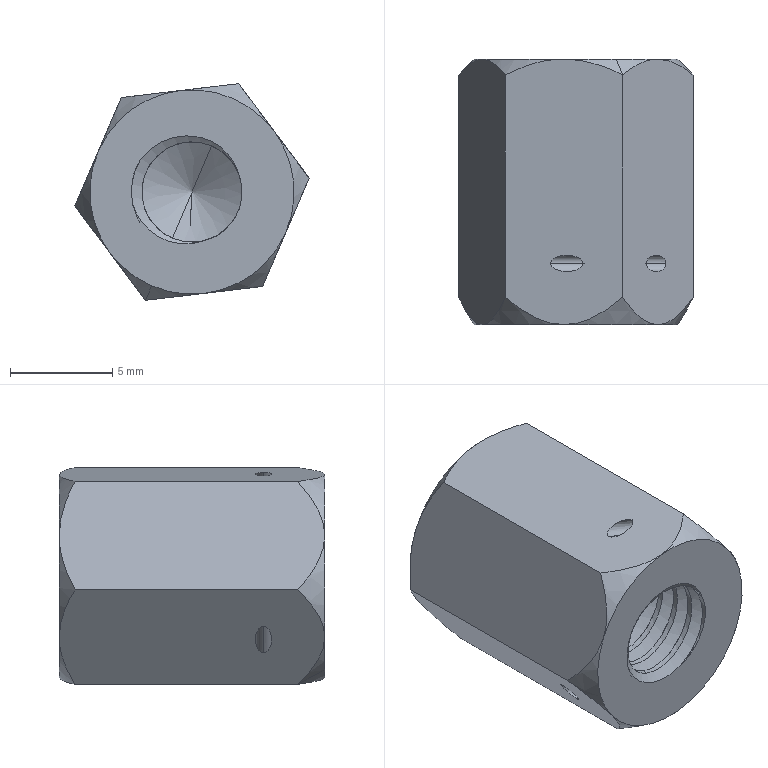Part | SolidWorks | features BaseBody 1 | 1 solid | 48 faces | box 11.466 x 13 x 10.611 mm | volume 869.633 mm3 | cylinder 20 | cone 16 | plane 9 | spline 3 | commonest cylinder face diameters 4.92 x16 0.8 x4